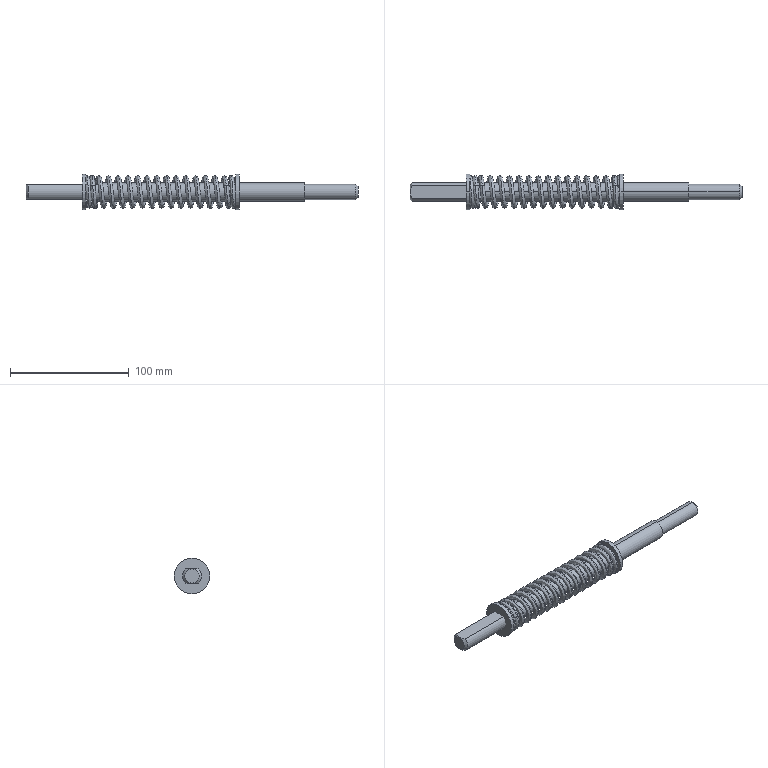Part | SolidWorks | features LayoutProfileFeature 1 | 4 solids | 53 faces | box 280 x 30 x 30 mm | volume 71173 mm3 | spline 22 | plane 15 | cylinder 12 | cone 4 | commonest cylinder face diameters 13 x6 30 x4 16 x2